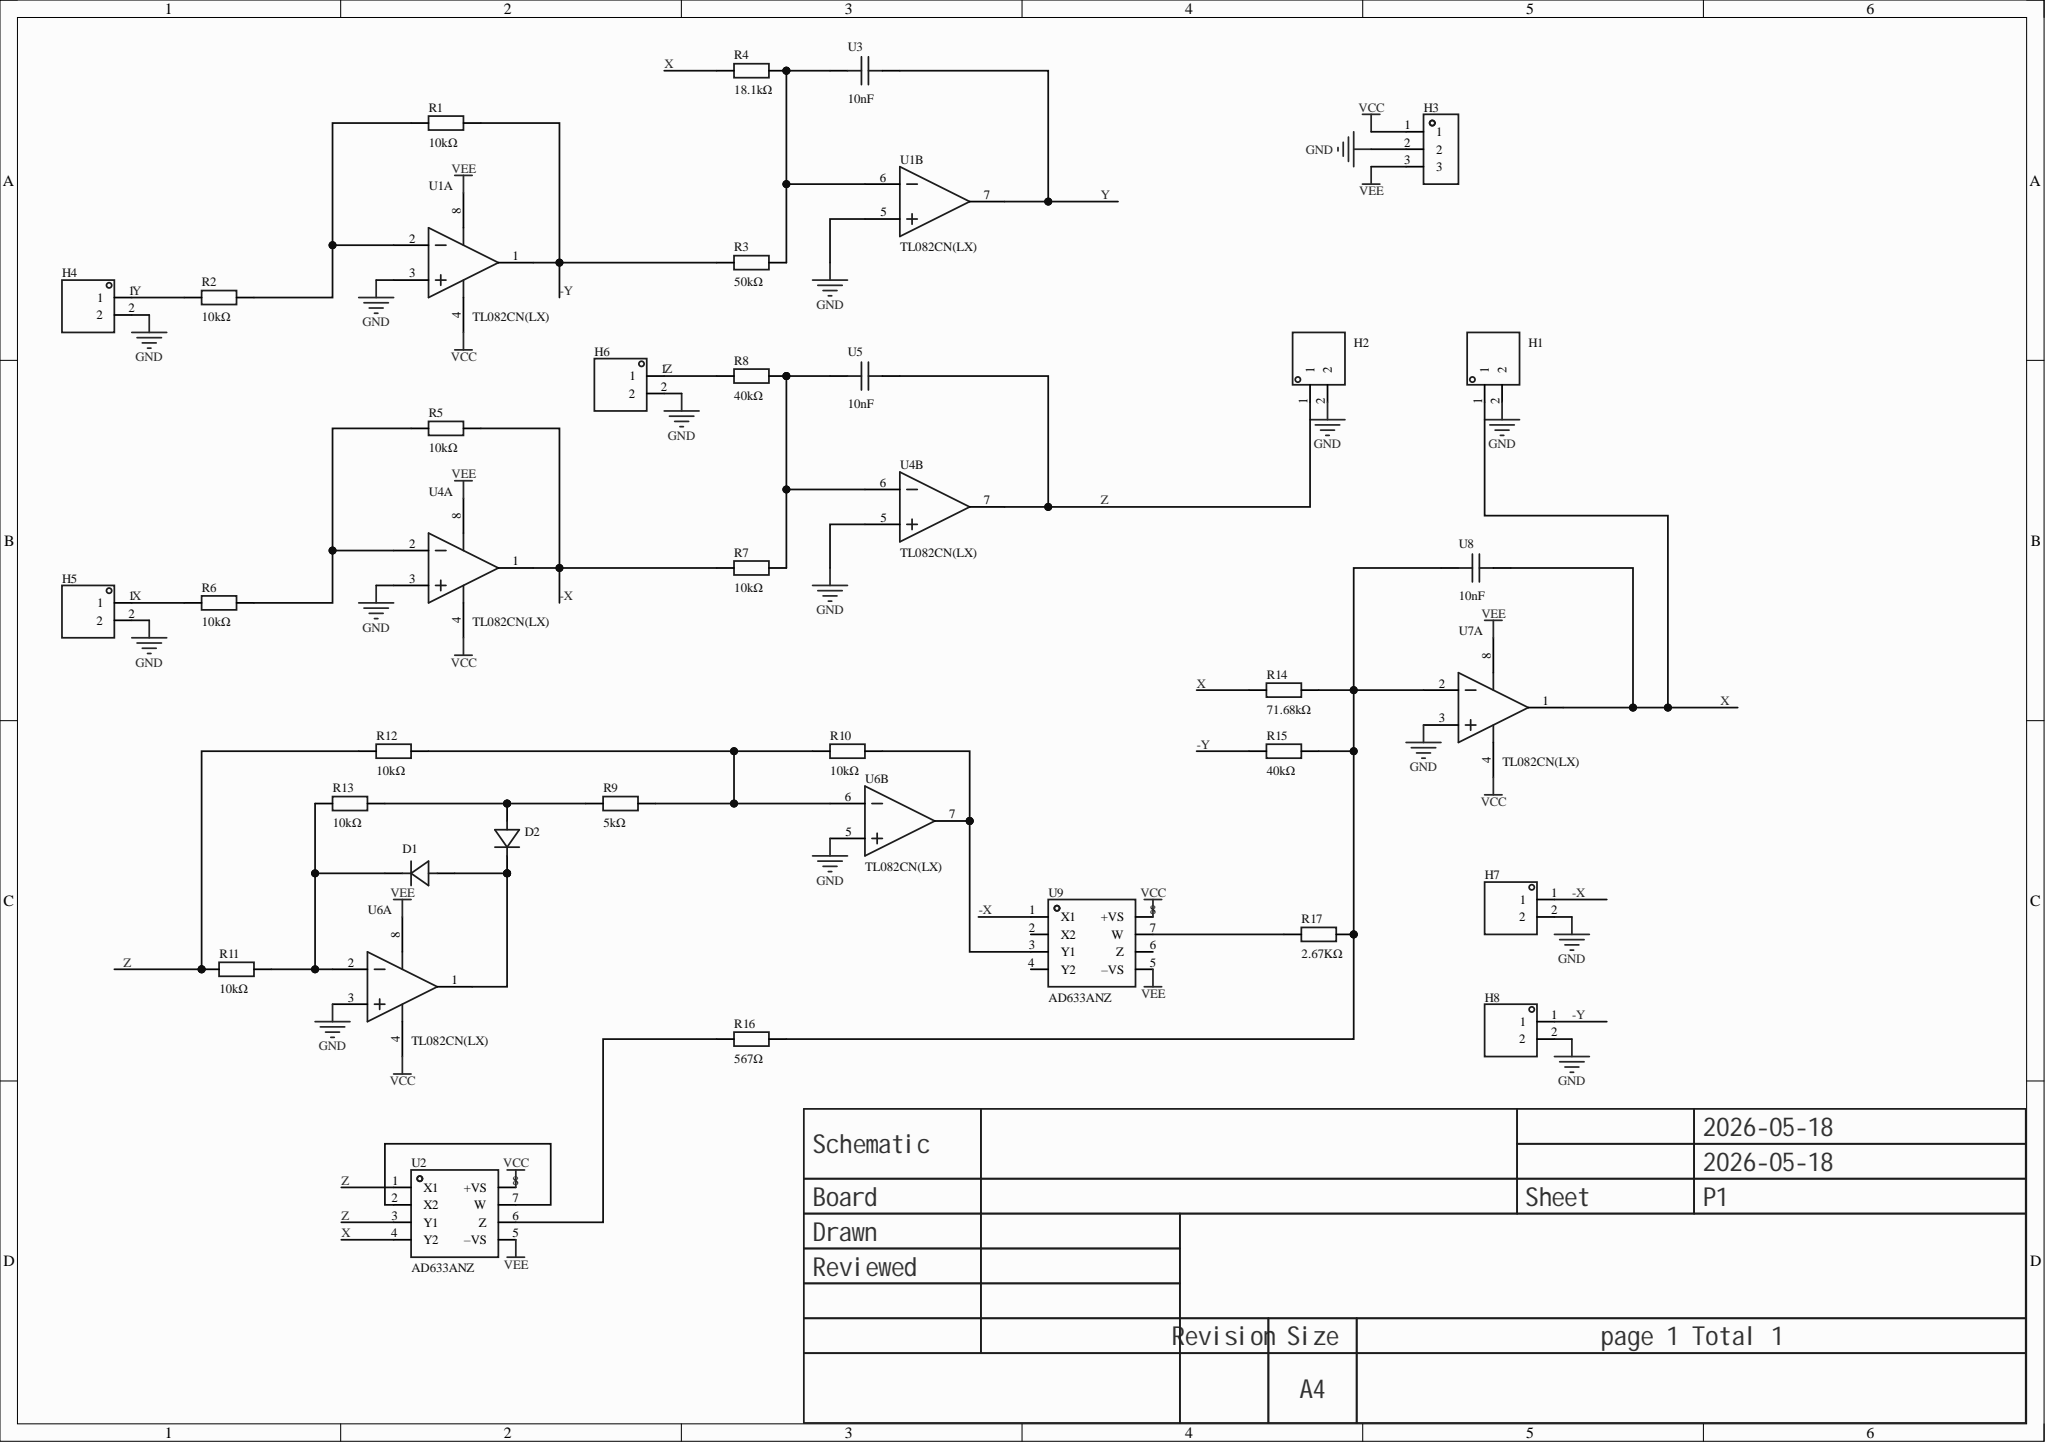Circuit board | Altium Designer | 36 parts | 21 nets
Bill of materials:
Comment,Description,Designator,Footprint,LibRef,Quantity
"","","D1, D2","DO_1N4007","D_1N4007A","2"
"","","H1, H2, H4, H5, H6, H7, H8","HDR-TH_2P-P2.54-V-M-1","HDR-M_2.54_1x2P","7"
"","","H3","HDR-TH_3P-P2.54-V-M","HDR-M_2.54_1x3P","1"
"10kΩ","","R1, R2, R5, R6, R7, R10, R11, R12, R13","Res_1/8W","Res_AXIAL-1/8W","9"
"50kΩ","","R3","Res_1/8W","Res_AXIAL-1/8W","1"
"18.1kΩ","","R4","Res_1/8W","Res_AXIAL-1/8W","1"
"40kΩ","","R8, R15","Res_1/8W","Res_AXIAL-1/8W","2"
"5kΩ","","R9","Res_1/8W","Res_AXIAL-1/8W","1"
"71.68kΩ","","R14","Res_1/8W","Res_AXIAL-1/8W","1"
"567Ω","","R16","Res_1/8W","Res_AXIAL-1/8W","1"
"2.67KΩ","","R17","Res_1/8W","Res_AXIAL-1/8W","1"
"TL082CN(LX)","Amplifier count: 2; gain-bandwidth product (GBW): 1.3MHz; input offset voltage (Vos): 2mV; slew rate (SR): 14V/us; input bias current (Ib): 30pA;","U1, U4, U6, U7","PDIP-8_L9.6-W6.4-P2.54-LS7.6-BL","TL082CN(LX)","4"
"AD633ANZ","Quadrant: four-quadrant; slew rate (SR): 20V/us; bandwidth: 1MHz;","U2, U9","PDIP-8_L9.3-W6.4-P2.54-LS7.9-BL-1","AD633ANZ","2"
"10nF","","U3, U5, U8","CAP-TH_L5.0-W2.5-P5.00-D1.0","100nF","3"
Netlist (Protel format):
[
D1
DO_1N4007




]
[
D2
DO_1N4007




]
[
H1
HDR-TH_2P-P2.54-V-M-1




]
[
H2
HDR-TH_2P-P2.54-V-M-1




]
[
H3
HDR-TH_3P-P2.54-V-M




]
[
H4
HDR-TH_2P-P2.54-V-M-1




]
[
H5
HDR-TH_2P-P2.54-V-M-1




]
[
H6
HDR-TH_2P-P2.54-V-M-1




]
[
H7
HDR-TH_2P-P2.54-V-M-1




]
[
H8
HDR-TH_2P-P2.54-V-M-1




]
[
R1
Res_1/8W
10kΩ



]
[
R2
Res_1/8W
10kΩ



]
[
R3
Res_1/8W
50kΩ



]
[
R4
Res_1/8W
18.1kΩ



]
[
R5
Res_1/8W
10kΩ



]
[
R6
Res_1/8W
10kΩ



]
[
R7
Res_1/8W
10kΩ



]
[
R8
Res_1/8W
40kΩ



]
[
R9
Res_1/8W
5kΩ



]
[
R10
Res_1/8W
10kΩ



]
[
R11
Res_1/8W
10kΩ



]
[
R12
Res_1/8W
10kΩ



]
[
R13
Res_1/8W
10kΩ



]
[
R14
Res_1/8W
71.68kΩ



]
[
R15
Res_1/8W
40kΩ



]
[
R16
Res_1/8W
567Ω



]
[
R17
Res_1/8W
2.67KΩ



]
[
U1
PDIP-8_L9.6-W6.4-P2.54-LS7.6-BL
TL082CN(LX)



]
[
U2
PDIP-8_L9.3-W6.4-P2.54-LS7.9-BL-1
AD633ANZ



]
[
U3
CAP-TH_L5.0-W2.5-P5.00-D1.0
10nF



]
[
U4
PDIP-8_L9.6-W6.4-P2.54-LS7.6-BL
TL082CN(LX)



]
[
U5
CAP-TH_L5.0-W2.5-P5.00-D1.0
10nF



]
[
U6
PDIP-8_L9.6-W6.4-P2.54-LS7.6-BL
TL082CN(LX)



]
[
U7
PDIP-8_L9.6-W6.4-P2.54-LS7.6-BL
TL082CN(LX)



]
[
U8
CAP-TH_L5.0-W2.5-P5.00-D1.0
10nF



]
[
U9
PDIP-8_L9.3-W6.4-P2.54-LS7.9-BL-1
AD633ANZ



]
(
Z
H2-1
H6-1
R8-1
R11-1
R12-1
U2-1
U2-3
U4-7
U5-1
)
(
Y
H4-1
R2-1
U1-7
U3-1
)
(
X
H1-1
H5-1
R4-1
R6-1
R14-1
U2-4
U7-1
U8-1
)
(
VEE
H3-3
U1-8
U2-5
U4-8
U6-8
U7-8
U9-5
)
(
VCC
H3-1
U1-4
U2-8
U4-4
U6-4
U7-4
U9-8
)
(
NetU2_2
U2-2
U2-7
)
(
NetR17_1
R17-1
U9-7
)
(
NetR16_1
R16-1
U2-6
)
(
NetR14_2
R14-2
R15-2
R16-2
R17-2
U7-2
U8-2
)
(
NetR10_2
R10-2
U6-7
U9-3
)
(
NetR9_2
R9-2
R10-1
R12-2
U6-6
)
(
NetR7_2
R7-2
R8-2
U4-6
U5-2
)
(
NetR5_1
R5-1
R6-2
U4-2
)
(
NetR3_2
R3-2
R4-2
U1-6
U3-2
)
(
NetR1_1
R1-1
R2-2
U1-2
)
(
NetD2_2
D2-2
R9-1
R13-2
)
(
NetD1_2
D1-2
D2-1
U6-1
)
(
NetD1_1
D1-1
R11-2
R13-1
U6-2
)
(
GND
H1-2
H2-2
H3-2
H4-2
H5-2
H6-2
H7-2
H8-2
U1-3
U1-5
U4-3
U4-5
U6-3
U6-5
U7-3
)
(
-Y
H8-1
R1-2
R3-1
R15-1
U1-1
)
(
-X
H7-1
R5-2
R7-1
U4-1
U9-1
)